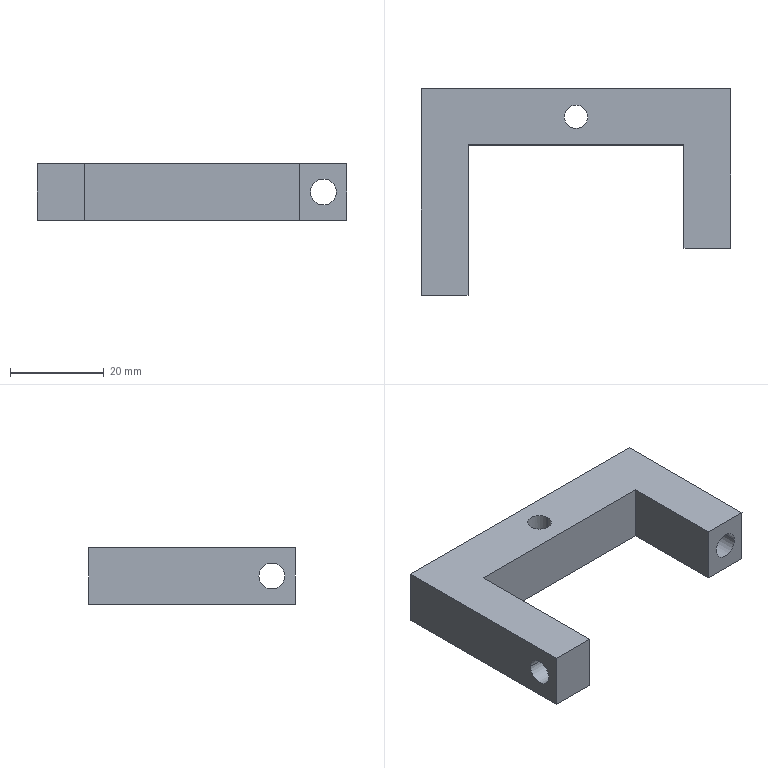Part | NX | 1 solid | 18 faces | box 65.997 x 44 x 12 mm | volume 14698 mm3 | plane 10 | cylinder 6 | cone 2 | commonest cylinder face diameters 5.5 x4 5 x2
STEP:
#1=CARTESIAN_POINT('',(1249.566,150.5,11.862));
#2=VERTEX_POINT('',#1);
#3=CARTESIAN_POINT('',(1249.566,116.5,11.862));
#4=VERTEX_POINT('',#3);
#5=CARTESIAN_POINT('',(1249.566,141.5,11.862));
#6=DIRECTION('',(0.,-1.,0.));
#7=VECTOR('',#6,1000.);
#8=LINE('',#5,#7);
#9=EDGE_CURVE('',#2,#4,#8,.T.);
#10=ORIENTED_EDGE('',*,*,#9,.F.);
#11=CARTESIAN_POINT('',(1249.566,150.5,23.862));
#12=VERTEX_POINT('',#11);
#13=CARTESIAN_POINT('',(1249.566,150.5,-7.371));
#14=DIRECTION('',(0.,0.,-1.));
#15=VECTOR('',#14,1000.);
#16=LINE('',#13,#15);
#17=EDGE_CURVE('',#12,#2,#16,.T.);
#18=ORIENTED_EDGE('',*,*,#17,.F.);
#19=CARTESIAN_POINT('',(1249.566,116.5,23.862));
#20=VERTEX_POINT('',#19);
#21=CARTESIAN_POINT('',(1249.566,141.5,23.862));
#22=DIRECTION('',(0.,1.,0.));
#23=VECTOR('',#22,1000.);
#24=LINE('',#21,#23);
#25=EDGE_CURVE('',#20,#12,#24,.T.);
#26=ORIENTED_EDGE('',*,*,#25,.F.);
#27=CARTESIAN_POINT('',(1249.566,116.5,-7.371));
#28=DIRECTION('',(0.,0.,1.));
#29=VECTOR('',#28,1000.);
#30=LINE('',#27,#29);
#31=EDGE_CURVE('',#4,#20,#30,.T.);
#32=ORIENTED_EDGE('',*,*,#31,.F.);
#33=EDGE_LOOP('',(#10,#18,#26,#32));
#34=FACE_BOUND('',#33,.T.);
#35=CARTESIAN_POINT('',(1249.566,141.5,12.862));
#36=DIRECTION('',(1.,0.,0.));
#37=DIRECTION('',(0.,-1.,0.));
#38=AXIS2_PLACEMENT_3D('',#35,#36,#37);
#39=PLANE('',#38);
#40=ADVANCED_FACE('',(#34),#39,.T.);
#41=ORIENTED_EDGE('',*,*,#31,.T.);
#42=CARTESIAN_POINT('',(1239.566,116.5,23.862));
#43=VERTEX_POINT('',#42);
#44=CARTESIAN_POINT('',(1214.351,116.5,23.862));
#45=DIRECTION('',(1.,0.,0.));
#46=VECTOR('',#45,1000.);
#47=LINE('',#44,#46);
#48=EDGE_CURVE('',#43,#20,#47,.T.);
#49=ORIENTED_EDGE('',*,*,#48,.F.);
#50=CARTESIAN_POINT('',(1239.566,116.5,11.862));
#51=VERTEX_POINT('',#50);
#52=CARTESIAN_POINT('',(1239.566,116.5,-7.371));
#53=DIRECTION('',(0.,0.,1.));
#54=VECTOR('',#53,1000.);
#55=LINE('',#52,#54);
#56=EDGE_CURVE('',#51,#43,#55,.T.);
#57=ORIENTED_EDGE('',*,*,#56,.F.);
#58=CARTESIAN_POINT('',(1214.351,116.5,11.862));
#59=DIRECTION('',(-1.,0.,0.));
#60=VECTOR('',#59,1000.);
#61=LINE('',#58,#60);
#62=EDGE_CURVE('',#4,#51,#61,.T.);
#63=ORIENTED_EDGE('',*,*,#62,.F.);
#64=EDGE_LOOP('',(#41,#49,#57,#63));
#65=FACE_BOUND('',#64,.T.);
#66=CARTESIAN_POINT('',(1247.316,116.5,17.862));
#67=VERTEX_POINT('',#66);
#68=CARTESIAN_POINT('',(1241.816,116.5,17.862));
#69=VERTEX_POINT('',#68);
#70=CARTESIAN_POINT('',(1244.566,116.5,17.862));
#71=DIRECTION('',(0.,1.,0.));
#72=DIRECTION('',(-1.,0.,0.));
#73=AXIS2_PLACEMENT_3D('',#70,#71,#72);
#74=CIRCLE('',#73,2.75);
#75=EDGE_CURVE('',#67,#69,#74,.T.);
#76=ORIENTED_EDGE('',*,*,#75,.T.);
#77=CARTESIAN_POINT('',(1244.566,116.5,17.862));
#78=DIRECTION('',(0.,1.,0.));
#79=DIRECTION('',(-1.,0.,0.));
#80=AXIS2_PLACEMENT_3D('',#77,#78,#79);
#81=CIRCLE('',#80,2.75);
#82=EDGE_CURVE('',#69,#67,#81,.T.);
#83=ORIENTED_EDGE('',*,*,#82,.T.);
#84=EDGE_LOOP('',(#76,#83));
#85=FACE_BOUND('',#84,.T.);
#86=CARTESIAN_POINT('',(1244.599,116.5,17.969));
#87=DIRECTION('',(0.,-1.,0.));
#88=DIRECTION('',(0.,0.,-1.));
#89=AXIS2_PLACEMENT_3D('',#86,#87,#88);
#90=PLANE('',#89);
#91=ADVANCED_FACE('',(#65,#85),#90,.T.);
#92=CARTESIAN_POINT('',(1183.569,150.5,23.862));
#93=VERTEX_POINT('',#92);
#94=CARTESIAN_POINT('',(1183.569,106.5,23.862));
#95=VERTEX_POINT('',#94);
#96=CARTESIAN_POINT('',(1183.569,141.5,23.862));
#97=DIRECTION('',(0.,-1.,0.));
#98=VECTOR('',#97,1000.);
#99=LINE('',#96,#98);
#100=EDGE_CURVE('',#93,#95,#99,.T.);
#101=ORIENTED_EDGE('',*,*,#100,.F.);
#102=CARTESIAN_POINT('',(1183.569,150.5,11.862));
#103=VERTEX_POINT('',#102);
#104=CARTESIAN_POINT('',(1183.569,150.5,-7.371));
#105=DIRECTION('',(0.,0.,-1.));
#106=VECTOR('',#105,1000.);
#107=LINE('',#104,#106);
#108=EDGE_CURVE('',#93,#103,#107,.T.);
#109=ORIENTED_EDGE('',*,*,#108,.T.);
#110=CARTESIAN_POINT('',(1183.569,106.5,11.862));
#111=VERTEX_POINT('',#110);
#112=CARTESIAN_POINT('',(1183.569,141.5,11.862));
#113=DIRECTION('',(0.,1.,0.));
#114=VECTOR('',#113,1000.);
#115=LINE('',#112,#114);
#116=EDGE_CURVE('',#111,#103,#115,.T.);
#117=ORIENTED_EDGE('',*,*,#116,.F.);
#118=CARTESIAN_POINT('',(1183.569,106.5,-7.371));
#119=DIRECTION('',(0.,0.,1.));
#120=VECTOR('',#119,1000.);
#121=LINE('',#118,#120);
#122=EDGE_CURVE('',#111,#95,#121,.T.);
#123=ORIENTED_EDGE('',*,*,#122,.T.);
#124=EDGE_LOOP('',(#101,#109,#117,#123));
#125=FACE_BOUND('',#124,.T.);
#126=CARTESIAN_POINT('',(1183.569,108.75,17.862));
#127=VERTEX_POINT('',#126);
#128=CARTESIAN_POINT('',(1183.569,114.25,17.862));
#129=VERTEX_POINT('',#128);
#130=CARTESIAN_POINT('',(1183.569,111.5,17.862));
#131=DIRECTION('',(-1.,0.,0.));
#132=DIRECTION('',(0.,1.,0.));
#133=AXIS2_PLACEMENT_3D('',#130,#131,#132);
#134=CIRCLE('',#133,2.75);
#135=EDGE_CURVE('',#127,#129,#134,.T.);
#136=ORIENTED_EDGE('',*,*,#135,.F.);
#137=CARTESIAN_POINT('',(1183.569,111.5,17.862));
#138=DIRECTION('',(-1.,0.,0.));
#139=DIRECTION('',(0.,1.,0.));
#140=AXIS2_PLACEMENT_3D('',#137,#138,#139);
#141=CIRCLE('',#140,2.75);
#142=EDGE_CURVE('',#129,#127,#141,.T.);
#143=ORIENTED_EDGE('',*,*,#142,.F.);
#144=EDGE_LOOP('',(#136,#143));
#145=FACE_BOUND('',#144,.T.);
#146=CARTESIAN_POINT('',(1183.569,141.5,22.853));
#147=DIRECTION('',(-1.,0.,0.));
#148=DIRECTION('',(0.,0.,1.));
#149=AXIS2_PLACEMENT_3D('',#146,#147,#148);
#150=PLANE('',#149);
#151=ADVANCED_FACE('',(#125,#145),#150,.T.);
#152=CARTESIAN_POINT('',(1193.569,106.5,11.862));
#153=VERTEX_POINT('',#152);
#154=CARTESIAN_POINT('',(1193.569,106.5,23.862));
#155=VERTEX_POINT('',#154);
#156=CARTESIAN_POINT('',(1193.569,106.5,-7.371));
#157=DIRECTION('',(0.,0.,1.));
#158=VECTOR('',#157,1000.);
#159=LINE('',#156,#158);
#160=EDGE_CURVE('',#153,#155,#159,.T.);
#161=ORIENTED_EDGE('',*,*,#160,.T.);
#162=CARTESIAN_POINT('',(1214.351,106.5,23.862));
#163=DIRECTION('',(1.,0.,0.));
#164=VECTOR('',#163,1000.);
#165=LINE('',#162,#164);
#166=EDGE_CURVE('',#95,#155,#165,.T.);
#167=ORIENTED_EDGE('',*,*,#166,.F.);
#168=ORIENTED_EDGE('',*,*,#122,.F.);
#169=CARTESIAN_POINT('',(1214.351,106.5,11.862));
#170=DIRECTION('',(-1.,0.,0.));
#171=VECTOR('',#170,1000.);
#172=LINE('',#169,#171);
#173=EDGE_CURVE('',#153,#111,#172,.T.);
#174=ORIENTED_EDGE('',*,*,#173,.F.);
#175=EDGE_LOOP('',(#161,#167,#168,#174));
#176=FACE_BOUND('',#175,.T.);
#177=CARTESIAN_POINT('',(1244.599,106.5,17.969));
#178=DIRECTION('',(0.,-1.,0.));
#179=DIRECTION('',(0.,0.,-1.));
#180=AXIS2_PLACEMENT_3D('',#177,#178,#179);
#181=PLANE('',#180);
#182=ADVANCED_FACE('',(#176),#181,.T.);
#183=ORIENTED_EDGE('',*,*,#75,.F.);
#184=CARTESIAN_POINT('',(1247.316,150.5,17.862));
#185=VERTEX_POINT('',#184);
#186=CARTESIAN_POINT('',(1247.316,113.1,17.862));
#187=DIRECTION('',(0.,1.,0.));
#188=VECTOR('',#187,1000.);
#189=LINE('',#186,#188);
#190=EDGE_CURVE('',#67,#185,#189,.T.);
#191=ORIENTED_EDGE('',*,*,#190,.T.);
#192=CARTESIAN_POINT('',(1241.816,150.5,17.862));
#193=VERTEX_POINT('',#192);
#194=CARTESIAN_POINT('',(1244.566,150.5,17.862));
#195=DIRECTION('',(0.,1.,0.));
#196=DIRECTION('',(-1.,0.,0.));
#197=AXIS2_PLACEMENT_3D('',#194,#195,#196);
#198=CIRCLE('',#197,2.75);
#199=EDGE_CURVE('',#185,#193,#198,.T.);
#200=ORIENTED_EDGE('',*,*,#199,.T.);
#201=CARTESIAN_POINT('',(1241.816,113.1,17.862));
#202=DIRECTION('',(0.,1.,0.));
#203=VECTOR('',#202,1000.);
#204=LINE('',#201,#203);
#205=EDGE_CURVE('',#69,#193,#204,.T.);
#206=ORIENTED_EDGE('',*,*,#205,.F.);
#207=EDGE_LOOP('',(#183,#191,#200,#206));
#208=FACE_BOUND('',#207,.T.);
#209=CARTESIAN_POINT('',(1244.566,113.1,17.862));
#210=DIRECTION('',(0.,1.,0.));
#211=DIRECTION('',(-1.,0.,0.));
#212=AXIS2_PLACEMENT_3D('',#209,#210,#211);
#213=CYLINDRICAL_SURFACE('',#212,2.75);
#214=ADVANCED_FACE('',(#208),#213,.F.);
#215=ORIENTED_EDGE('',*,*,#135,.T.);
#216=CARTESIAN_POINT('',(1193.569,114.25,17.862));
#217=VERTEX_POINT('',#216);
#218=CARTESIAN_POINT('',(1259.766,114.25,17.862));
#219=DIRECTION('',(-1.,0.,0.));
#220=VECTOR('',#219,1000.);
#221=LINE('',#218,#220);
#222=EDGE_CURVE('',#217,#129,#221,.T.);
#223=ORIENTED_EDGE('',*,*,#222,.F.);
#224=CARTESIAN_POINT('',(1193.569,108.75,17.862));
#225=VERTEX_POINT('',#224);
#226=CARTESIAN_POINT('',(1193.569,111.5,17.862));
#227=DIRECTION('',(-1.,0.,0.));
#228=DIRECTION('',(0.,1.,0.));
#229=AXIS2_PLACEMENT_3D('',#226,#227,#228);
#230=CIRCLE('',#229,2.75);
#231=EDGE_CURVE('',#225,#217,#230,.T.);
#232=ORIENTED_EDGE('',*,*,#231,.F.);
#233=CARTESIAN_POINT('',(1259.766,108.75,17.862));
#234=DIRECTION('',(-1.,0.,0.));
#235=VECTOR('',#234,1000.);
#236=LINE('',#233,#235);
#237=EDGE_CURVE('',#225,#127,#236,.T.);
#238=ORIENTED_EDGE('',*,*,#237,.T.);
#239=EDGE_LOOP('',(#215,#223,#232,#238));
#240=FACE_BOUND('',#239,.T.);
#241=CARTESIAN_POINT('',(1259.766,111.5,17.862));
#242=DIRECTION('',(-1.,0.,0.));
#243=DIRECTION('',(0.,1.,0.));
#244=AXIS2_PLACEMENT_3D('',#241,#242,#243);
#245=CYLINDRICAL_SURFACE('',#244,2.75);
#246=ADVANCED_FACE('',(#240),#245,.F.);
#247=ORIENTED_EDGE('',*,*,#17,.T.);
#248=CARTESIAN_POINT('',(1214.351,150.5,11.862));
#249=DIRECTION('',(1.,0.,0.));
#250=VECTOR('',#249,1000.);
#251=LINE('',#248,#250);
#252=EDGE_CURVE('',#103,#2,#251,.T.);
#253=ORIENTED_EDGE('',*,*,#252,.F.);
#254=ORIENTED_EDGE('',*,*,#108,.F.);
#255=CARTESIAN_POINT('',(1214.351,150.5,23.862));
#256=DIRECTION('',(-1.,0.,0.));
#257=VECTOR('',#256,1000.);
#258=LINE('',#255,#257);
#259=EDGE_CURVE('',#12,#93,#258,.T.);
#260=ORIENTED_EDGE('',*,*,#259,.F.);
#261=EDGE_LOOP('',(#247,#253,#254,#260));
#262=FACE_BOUND('',#261,.T.);
#263=ORIENTED_EDGE('',*,*,#199,.F.);
#264=CARTESIAN_POINT('',(1244.566,150.5,17.862));
#265=DIRECTION('',(0.,1.,0.));
#266=DIRECTION('',(-1.,0.,0.));
#267=AXIS2_PLACEMENT_3D('',#264,#265,#266);
#268=CIRCLE('',#267,2.75);
#269=EDGE_CURVE('',#193,#185,#268,.T.);
#270=ORIENTED_EDGE('',*,*,#269,.F.);
#271=EDGE_LOOP('',(#263,#270));
#272=FACE_BOUND('',#271,.T.);
#273=CARTESIAN_POINT('',(1214.357,150.5,12.629));
#274=DIRECTION('',(0.,1.,0.));
#275=DIRECTION('',(0.,0.,-1.));
#276=AXIS2_PLACEMENT_3D('',#273,#274,#275);
#277=PLANE('',#276);
#278=ADVANCED_FACE('',(#262,#272),#277,.T.);
#279=CARTESIAN_POINT('',(1239.566,138.5,23.862));
#280=VERTEX_POINT('',#279);
#281=CARTESIAN_POINT('',(1239.566,138.5,11.862));
#282=VERTEX_POINT('',#281);
#283=CARTESIAN_POINT('',(1239.566,138.5,-7.371));
#284=DIRECTION('',(0.,0.,-1.));
#285=VECTOR('',#284,1000.);
#286=LINE('',#283,#285);
#287=EDGE_CURVE('',#280,#282,#286,.T.);
#288=ORIENTED_EDGE('',*,*,#287,.F.);
#289=CARTESIAN_POINT('',(1193.569,138.5,23.862));
#290=VERTEX_POINT('',#289);
#291=CARTESIAN_POINT('',(1214.351,138.5,23.862));
#292=DIRECTION('',(-1.,0.,0.));
#293=VECTOR('',#292,1000.);
#294=LINE('',#291,#293);
#295=EDGE_CURVE('',#280,#290,#294,.T.);
#296=ORIENTED_EDGE('',*,*,#295,.T.);
#297=CARTESIAN_POINT('',(1193.569,138.5,11.862));
#298=VERTEX_POINT('',#297);
#299=CARTESIAN_POINT('',(1193.569,138.5,-7.371));
#300=DIRECTION('',(0.,0.,-1.));
#301=VECTOR('',#300,1000.);
#302=LINE('',#299,#301);
#303=EDGE_CURVE('',#290,#298,#302,.T.);
#304=ORIENTED_EDGE('',*,*,#303,.T.);
#305=CARTESIAN_POINT('',(1214.351,138.5,11.862));
#306=DIRECTION('',(1.,0.,0.));
#307=VECTOR('',#306,1000.);
#308=LINE('',#305,#307);
#309=EDGE_CURVE('',#298,#282,#308,.T.);
#310=ORIENTED_EDGE('',*,*,#309,.T.);
#311=EDGE_LOOP('',(#288,#296,#304,#310));
#312=FACE_BOUND('',#311,.T.);
#313=CARTESIAN_POINT('',(1214.357,138.5,12.629));
#314=DIRECTION('',(0.,1.,0.));
#315=DIRECTION('',(0.,0.,-1.));
#316=AXIS2_PLACEMENT_3D('',#313,#314,#315);
#317=PLANE('',#316);
#318=ADVANCED_FACE('',(#312),#317,.F.);
#319=CARTESIAN_POINT('',(1193.569,141.5,11.862));
#320=DIRECTION('',(0.,-1.,0.));
#321=VECTOR('',#320,1000.);
#322=LINE('',#319,#321);
#323=EDGE_CURVE('',#298,#153,#322,.T.);
#324=ORIENTED_EDGE('',*,*,#323,.T.);
#325=ORIENTED_EDGE('',*,*,#173,.T.);
#326=ORIENTED_EDGE('',*,*,#116,.T.);
#327=ORIENTED_EDGE('',*,*,#252,.T.);
#328=ORIENTED_EDGE('',*,*,#9,.T.);
#329=ORIENTED_EDGE('',*,*,#62,.T.);
#330=CARTESIAN_POINT('',(1239.566,141.5,11.862));
#331=DIRECTION('',(0.,1.,0.));
#332=VECTOR('',#331,1000.);
#333=LINE('',#330,#332);
#334=EDGE_CURVE('',#51,#282,#333,.T.);
#335=ORIENTED_EDGE('',*,*,#334,.T.);
#336=ORIENTED_EDGE('',*,*,#309,.F.);
#337=EDGE_LOOP('',(#324,#325,#326,#327,#328,#329,#335,#336));
#338=FACE_BOUND('',#337,.T.);
#339=CARTESIAN_POINT('',(1216.568,141.05,11.862));
#340=VERTEX_POINT('',#339);
#341=CARTESIAN_POINT('',(1216.568,147.95,11.862));
#342=VERTEX_POINT('',#341);
#343=CARTESIAN_POINT('',(1216.568,144.5,11.862));
#344=DIRECTION('',(0.,0.,-1.));
#345=DIRECTION('',(1.,0.,0.));
#346=AXIS2_PLACEMENT_3D('',#343,#344,#345);
#347=CIRCLE('',#346,3.45);
#348=EDGE_CURVE('',#340,#342,#347,.T.);
#349=ORIENTED_EDGE('',*,*,#348,.F.);
#350=CARTESIAN_POINT('',(1216.568,144.5,11.862));
#351=DIRECTION('',(0.,0.,-1.));
#352=DIRECTION('',(1.,0.,0.));
#353=AXIS2_PLACEMENT_3D('',#350,#351,#352);
#354=CIRCLE('',#353,3.45);
#355=EDGE_CURVE('',#342,#340,#354,.T.);
#356=ORIENTED_EDGE('',*,*,#355,.F.);
#357=EDGE_LOOP('',(#349,#356));
#358=FACE_BOUND('',#357,.T.);
#359=CARTESIAN_POINT('',(1192.569,141.5,11.862));
#360=DIRECTION('',(0.,0.,-1.));
#361=DIRECTION('',(-1.,0.,0.));
#362=AXIS2_PLACEMENT_3D('',#359,#360,#361);
#363=PLANE('',#362);
#364=ADVANCED_FACE('',(#338,#358),#363,.T.);
#365=ORIENTED_EDGE('',*,*,#287,.T.);
#366=ORIENTED_EDGE('',*,*,#334,.F.);
#367=ORIENTED_EDGE('',*,*,#56,.T.);
#368=CARTESIAN_POINT('',(1239.566,141.5,23.862));
#369=DIRECTION('',(0.,1.,0.));
#370=VECTOR('',#369,1000.);
#371=LINE('',#368,#370);
#372=EDGE_CURVE('',#43,#280,#371,.T.);
#373=ORIENTED_EDGE('',*,*,#372,.T.);
#374=EDGE_LOOP('',(#365,#366,#367,#373));
#375=FACE_BOUND('',#374,.T.);
#376=CARTESIAN_POINT('',(1239.566,141.5,12.862));
#377=DIRECTION('',(-1.,0.,0.));
#378=DIRECTION('',(0.,0.,1.));
#379=AXIS2_PLACEMENT_3D('',#376,#377,#378);
#380=PLANE('',#379);
#381=ADVANCED_FACE('',(#375),#380,.T.);
#382=ORIENTED_EDGE('',*,*,#303,.F.);
#383=CARTESIAN_POINT('',(1193.569,141.5,23.862));
#384=DIRECTION('',(0.,1.,0.));
#385=VECTOR('',#384,1000.);
#386=LINE('',#383,#385);
#387=EDGE_CURVE('',#155,#290,#386,.T.);
#388=ORIENTED_EDGE('',*,*,#387,.F.);
#389=ORIENTED_EDGE('',*,*,#160,.F.);
#390=ORIENTED_EDGE('',*,*,#323,.F.);
#391=EDGE_LOOP('',(#382,#388,#389,#390));
#392=FACE_BOUND('',#391,.T.);
#393=CARTESIAN_POINT('',(1193.569,111.5,17.862));
#394=DIRECTION('',(-1.,0.,0.));
#395=DIRECTION('',(0.,1.,0.));
#396=AXIS2_PLACEMENT_3D('',#393,#394,#395);
#397=CIRCLE('',#396,2.75);
#398=EDGE_CURVE('',#217,#225,#397,.T.);
#399=ORIENTED_EDGE('',*,*,#398,.T.);
#400=ORIENTED_EDGE('',*,*,#231,.T.);
#401=EDGE_LOOP('',(#399,#400));
#402=FACE_BOUND('',#401,.T.);
#403=CARTESIAN_POINT('',(1193.569,141.5,22.853));
#404=DIRECTION('',(1.,0.,0.));
#405=DIRECTION('',(0.,-1.,0.));
#406=AXIS2_PLACEMENT_3D('',#403,#404,#405);
#407=PLANE('',#406);
#408=ADVANCED_FACE('',(#392,#402),#407,.T.);
#409=ORIENTED_EDGE('',*,*,#372,.F.);
#410=ORIENTED_EDGE('',*,*,#48,.T.);
#411=ORIENTED_EDGE('',*,*,#25,.T.);
#412=ORIENTED_EDGE('',*,*,#259,.T.);
#413=ORIENTED_EDGE('',*,*,#100,.T.);
#414=ORIENTED_EDGE('',*,*,#166,.T.);
#415=ORIENTED_EDGE('',*,*,#387,.T.);
#416=ORIENTED_EDGE('',*,*,#295,.F.);
#417=EDGE_LOOP('',(#409,#410,#411,#412,#413,#414,#415,#416));
#418=FACE_BOUND('',#417,.T.);
#419=CARTESIAN_POINT('',(1214.068,144.5,23.862));
#420=VERTEX_POINT('',#419);
#421=CARTESIAN_POINT('',(1219.068,144.5,23.862));
#422=VERTEX_POINT('',#421);
#423=CARTESIAN_POINT('',(1216.568,144.5,23.862));
#424=DIRECTION('',(0.,0.,-1.));
#425=DIRECTION('',(-1.,0.,0.));
#426=AXIS2_PLACEMENT_3D('',#423,#424,#425);
#427=CIRCLE('',#426,2.5);
#428=EDGE_CURVE('',#420,#422,#427,.T.);
#429=ORIENTED_EDGE('',*,*,#428,.T.);
#430=CARTESIAN_POINT('',(1216.568,144.5,23.862));
#431=DIRECTION('',(0.,0.,-1.));
#432=DIRECTION('',(-1.,0.,0.));
#433=AXIS2_PLACEMENT_3D('',#430,#431,#432);
#434=CIRCLE('',#433,2.5);
#435=EDGE_CURVE('',#422,#420,#434,.T.);
#436=ORIENTED_EDGE('',*,*,#435,.T.);
#437=EDGE_LOOP('',(#429,#436));
#438=FACE_BOUND('',#437,.T.);
#439=CARTESIAN_POINT('',(1248.195,112.64,23.862));
#440=DIRECTION('',(0.,0.,1.));
#441=DIRECTION('',(0.,-1.,0.));
#442=AXIS2_PLACEMENT_3D('',#439,#440,#441);
#443=PLANE('',#442);
#444=ADVANCED_FACE('',(#418,#438),#443,.T.);
#445=CARTESIAN_POINT('',(1216.568,142.,12.41));
#446=VERTEX_POINT('',#445);
#447=CARTESIAN_POINT('',(1214.068,144.5,12.41));
#448=VERTEX_POINT('',#447);
#449=CARTESIAN_POINT('',(1216.568,144.5,12.41));
#450=DIRECTION('',(0.,0.,-1.));
#451=DIRECTION('',(1.,0.,0.));
#452=AXIS2_PLACEMENT_3D('',#449,#450,#451);
#453=CIRCLE('',#452,2.5);
#454=EDGE_CURVE('',#446,#448,#453,.T.);
#455=ORIENTED_EDGE('',*,*,#454,.T.);
#456=CARTESIAN_POINT('',(1214.068,144.5,17.858));
#457=DIRECTION('',(0.,0.,-1.));
#458=VECTOR('',#457,1000.);
#459=LINE('',#456,#458);
#460=EDGE_CURVE('',#448,#420,#459,.F.);
#461=ORIENTED_EDGE('',*,*,#460,.T.);
#462=ORIENTED_EDGE('',*,*,#435,.F.);
#463=CARTESIAN_POINT('',(1219.068,144.5,12.41));
#464=VERTEX_POINT('',#463);
#465=CARTESIAN_POINT('',(1219.068,144.5,17.858));
#466=DIRECTION('',(0.,0.,-1.));
#467=VECTOR('',#466,1000.);
#468=LINE('',#465,#467);
#469=EDGE_CURVE('',#464,#422,#468,.F.);
#470=ORIENTED_EDGE('',*,*,#469,.F.);
#471=CARTESIAN_POINT('',(1216.568,144.5,12.41));
#472=DIRECTION('',(0.,0.,-1.));
#473=DIRECTION('',(1.,0.,0.));
#474=AXIS2_PLACEMENT_3D('',#471,#472,#473);
#475=CIRCLE('',#474,2.5);
#476=EDGE_CURVE('',#464,#446,#475,.T.);
#477=ORIENTED_EDGE('',*,*,#476,.T.);
#478=EDGE_LOOP('',(#455,#461,#462,#470,#477));
#479=FACE_BOUND('',#478,.T.);
#480=CARTESIAN_POINT('',(1216.568,144.5,17.858));
#481=DIRECTION('',(0.,0.,-1.));
#482=DIRECTION('',(-1.,0.,0.));
#483=AXIS2_PLACEMENT_3D('',#480,#481,#482);
#484=CYLINDRICAL_SURFACE('',#483,2.5);
#485=ADVANCED_FACE('',(#479),#484,.F.);
#486=ORIENTED_EDGE('',*,*,#454,.F.);
#487=CARTESIAN_POINT('',(1216.568,142.,12.41));
#488=DIRECTION('',(0.,-0.866,-0.5));
#489=VECTOR('',#488,1000.);
#490=LINE('',#487,#489);
#491=EDGE_CURVE('',#446,#340,#490,.T.);
#492=ORIENTED_EDGE('',*,*,#491,.T.);
#493=ORIENTED_EDGE('',*,*,#348,.T.);
#494=CARTESIAN_POINT('',(1216.568,147.,12.41));
#495=VERTEX_POINT('',#494);
#496=CARTESIAN_POINT('',(1216.568,147.,12.41));
#497=DIRECTION('',(0.,0.866,-0.5));
#498=VECTOR('',#497,1000.);
#499=LINE('',#496,#498);
#500=EDGE_CURVE('',#495,#342,#499,.T.);
#501=ORIENTED_EDGE('',*,*,#500,.F.);
#502=CARTESIAN_POINT('',(1216.568,144.5,12.41));
#503=DIRECTION('',(0.,0.,-1.));
#504=DIRECTION('',(1.,0.,0.));
#505=AXIS2_PLACEMENT_3D('',#502,#503,#504);
#506=CIRCLE('',#505,2.5);
#507=EDGE_CURVE('',#448,#495,#506,.T.);
#508=ORIENTED_EDGE('',*,*,#507,.F.);
#509=EDGE_LOOP('',(#486,#492,#493,#501,#508));
#510=FACE_BOUND('',#509,.T.);
#511=CARTESIAN_POINT('',(1216.568,144.5,12.41));
#512=DIRECTION('',(0.,0.,-1.));
#513=DIRECTION('',(0.,-1.,0.));
#514=AXIS2_PLACEMENT_3D('',#511,#512,#513);
#515=CONICAL_SURFACE('',#514,2.5,1.047);
#516=ADVANCED_FACE('',(#510),#515,.F.);
#517=ORIENTED_EDGE('',*,*,#428,.F.);
#518=ORIENTED_EDGE('',*,*,#460,.F.);
#519=ORIENTED_EDGE('',*,*,#507,.T.);
#520=CARTESIAN_POINT('',(1216.568,144.5,12.41));
#521=DIRECTION('',(0.,0.,-1.));
#522=DIRECTION('',(1.,0.,0.));
#523=AXIS2_PLACEMENT_3D('',#520,#521,#522);
#524=CIRCLE('',#523,2.5);
#525=EDGE_CURVE('',#495,#464,#524,.T.);
#526=ORIENTED_EDGE('',*,*,#525,.T.);
#527=ORIENTED_EDGE('',*,*,#469,.T.);
#528=EDGE_LOOP('',(#517,#518,#519,#526,#527));
#529=FACE_BOUND('',#528,.T.);
#530=CARTESIAN_POINT('',(1216.568,144.5,17.858));
#531=DIRECTION('',(0.,0.,-1.));
#532=DIRECTION('',(-1.,0.,0.));
#533=AXIS2_PLACEMENT_3D('',#530,#531,#532);
#534=CYLINDRICAL_SURFACE('',#533,2.5);
#535=ADVANCED_FACE('',(#529),#534,.F.);
#536=ORIENTED_EDGE('',*,*,#500,.T.);
#537=ORIENTED_EDGE('',*,*,#355,.T.);
#538=ORIENTED_EDGE('',*,*,#491,.F.);
#539=ORIENTED_EDGE('',*,*,#476,.F.);
#540=ORIENTED_EDGE('',*,*,#525,.F.);
#541=EDGE_LOOP('',(#536,#537,#538,#539,#540));
#542=FACE_BOUND('',#541,.T.);
#543=CARTESIAN_POINT('',(1216.568,144.5,12.41));
#544=DIRECTION('',(0.,0.,-1.));
#545=DIRECTION('',(0.,-1.,0.));
#546=AXIS2_PLACEMENT_3D('',#543,#544,#545);
#547=CONICAL_SURFACE('',#546,2.5,1.047);
#548=ADVANCED_FACE('',(#542),#547,.F.);
#549=ORIENTED_EDGE('',*,*,#398,.F.);
#550=ORIENTED_EDGE('',*,*,#222,.T.);
#551=ORIENTED_EDGE('',*,*,#142,.T.);
#552=ORIENTED_EDGE('',*,*,#237,.F.);
#553=EDGE_LOOP('',(#549,#550,#551,#552));
#554=FACE_BOUND('',#553,.T.);
#555=CARTESIAN_POINT('',(1259.766,111.5,17.862));
#556=DIRECTION('',(-1.,0.,0.));
#557=DIRECTION('',(0.,1.,0.));
#558=AXIS2_PLACEMENT_3D('',#555,#556,#557);
#559=CYLINDRICAL_SURFACE('',#558,2.75);
#560=ADVANCED_FACE('',(#554),#559,.F.);
#561=ORIENTED_EDGE('',*,*,#190,.F.);
#562=ORIENTED_EDGE('',*,*,#82,.F.);
#563=ORIENTED_EDGE('',*,*,#205,.T.);
#564=ORIENTED_EDGE('',*,*,#269,.T.);
#565=EDGE_LOOP('',(#561,#562,#563,#564));
#566=FACE_BOUND('',#565,.T.);
#567=CARTESIAN_POINT('',(1244.566,113.1,17.862));
#568=DIRECTION('',(0.,1.,0.));
#569=DIRECTION('',(-1.,0.,0.));
#570=AXIS2_PLACEMENT_3D('',#567,#568,#569);
#571=CYLINDRICAL_SURFACE('',#570,2.75);
#572=ADVANCED_FACE('',(#566),#571,.F.);
#573=CLOSED_SHELL('',(#40,#91,#151,#182,#214,#246,#278,#318,#364,#381,#408,#444,#485,#516,#535,#548,#560,#572));
#574=MANIFOLD_SOLID_BREP('',#573);
#575=(LENGTH_UNIT()NAMED_UNIT(*)SI_UNIT(.MILLI.,.METRE.));
#576=UNCERTAINTY_MEASURE_WITH_UNIT(LENGTH_MEASURE(0.00001),#575,'','');
#577=(NAMED_UNIT(*)PLANE_ANGLE_UNIT()SI_UNIT($,.RADIAN.));
#578=(NAMED_UNIT(*)SI_UNIT($,.STERADIAN.)SOLID_ANGLE_UNIT());
#579=(GEOMETRIC_REPRESENTATION_CONTEXT(3)GLOBAL_UNCERTAINTY_ASSIGNED_CONTEXT((#576))GLOBAL_UNIT_ASSIGNED_CONTEXT((#575,#577,#578))REPRESENTATION_CONTEXT('',''));
#580=ADVANCED_BREP_SHAPE_REPRESENTATION('',(#574),#579);